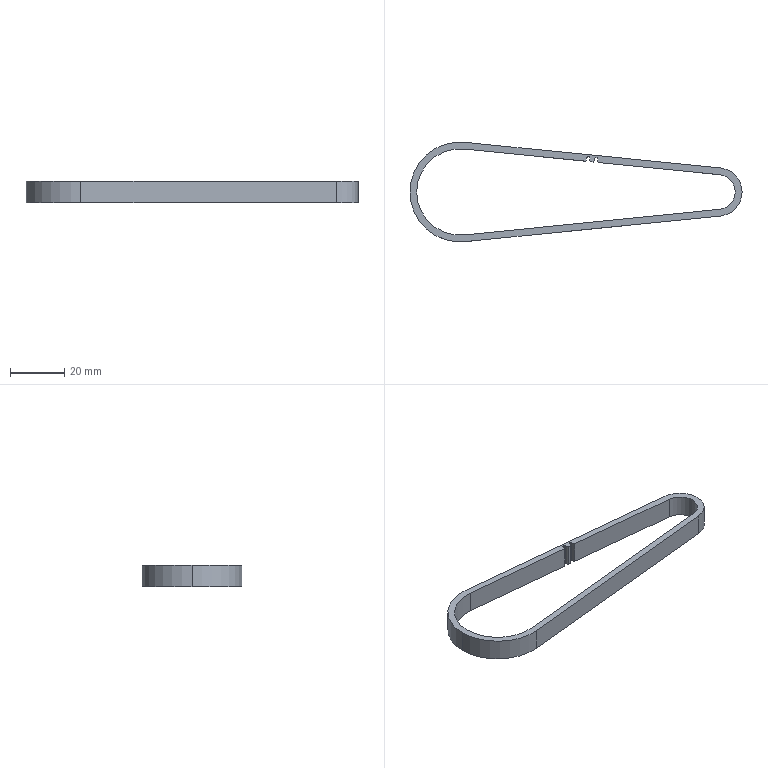Part | STEP file | 1 solid | 28 faces | box 122.93 x 36.98 x 8 mm | volume 5373 mm3 | cylinder 18 | plane 10 | commonest cylinder face diameters 0.6 x6 3.9 x4 0.2 x2 31.98 x2 36.98 x2 12.88 x1